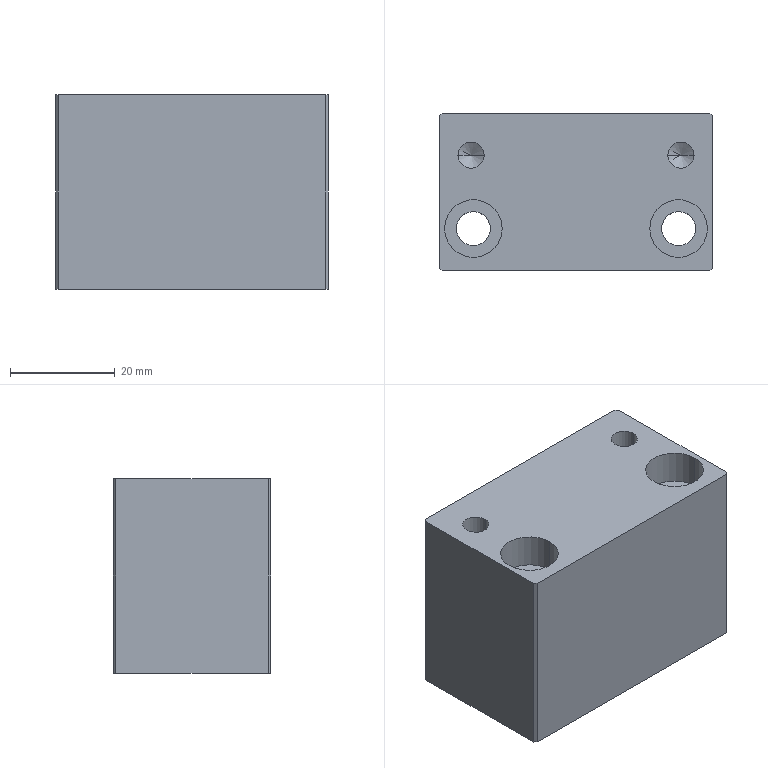Part | STEP file | spacer block 5 | 1 solid | 28 faces | box 52 x 30 x 37 mm | volume 53755 mm3 | cylinder 12 | plane 12 | cone 4 | commonest cylinder face diameters 5 x4 6.5 x4 11 x4